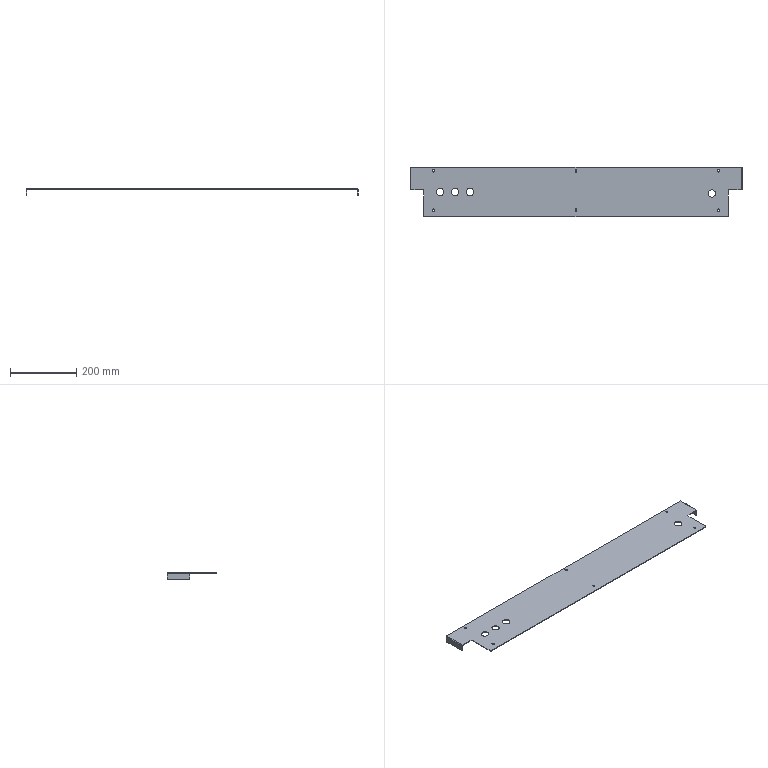Part | STEP file | Button Mounting Plate | 1 solid | 66 faces | box 1000 x 149 x 20 mm | volume 285929 mm3 | plane 34 | cylinder 32 | commonest cylinder face diameters 4.5 x12 6 x8 22.4 x6 0.2 x2 4.2 x2 22.5 x2